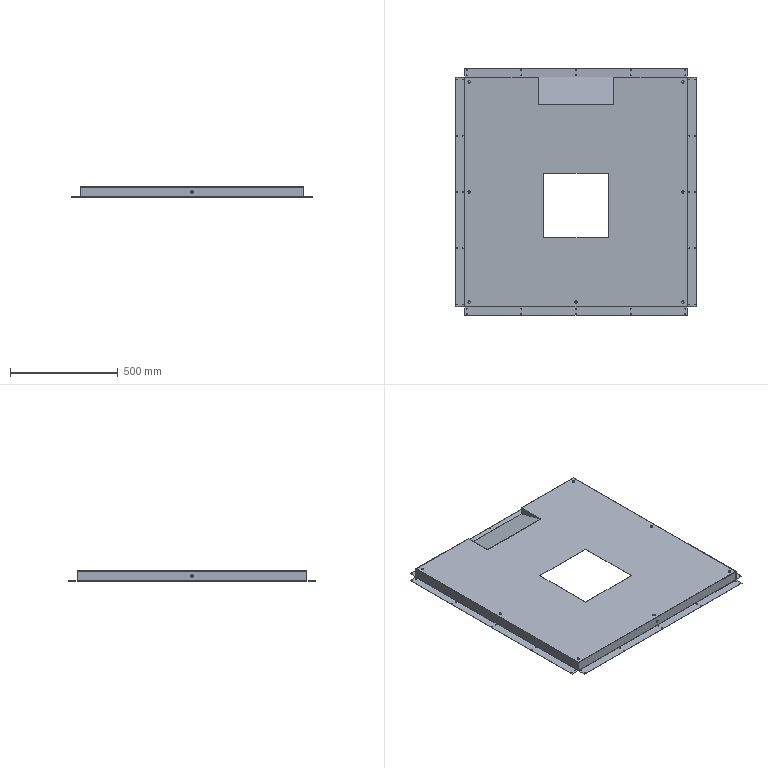Part | 2 solids | 204 faces | box 1113 x 1143 x 48 mm | volume 1362379 mm3 | cylinder 122 | plane 70 | spline 12 | commonest cylinder face diameters 4.2 x80 11 x14 0.4 x11 2.4 x11 10 x6